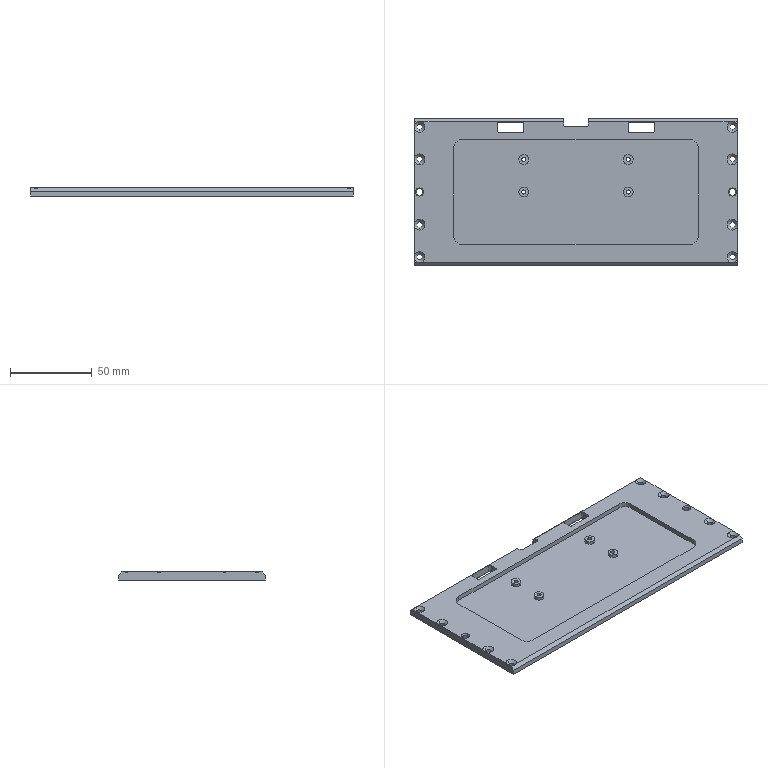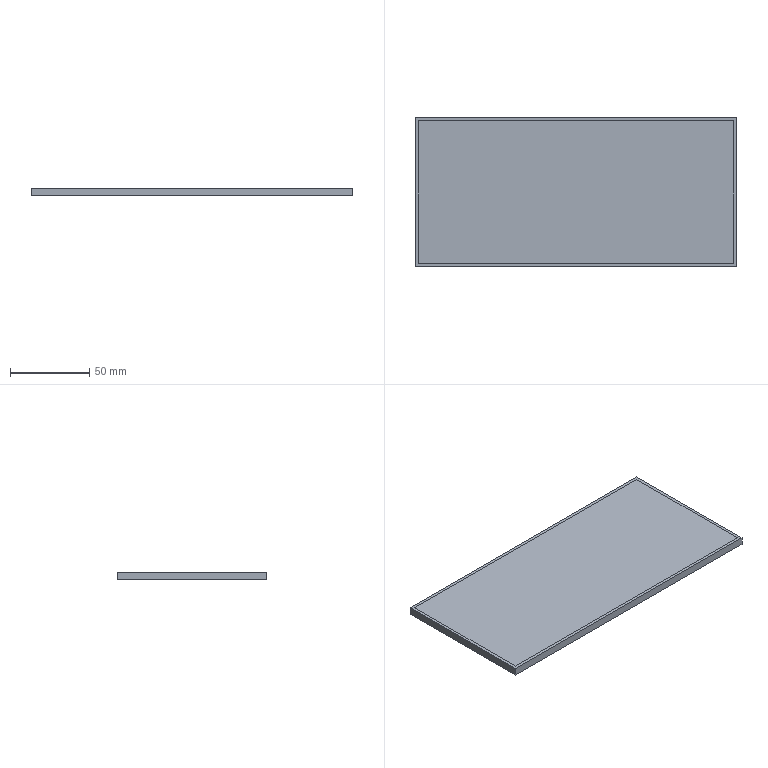CAM job | NX | 3-axis milling, drilling | part box 198 x 90 x 5 mm | stock box 202 x 94 x 5 mm
Tools:
number,name,description,diameter,corner_radius,flute_length,length,flutes
1,D6A45,Milling Tool-5 Parameters,6.0,0.0,50.0,75.0,2
16,3.4ZT,Drilling Tool,3.4,0.0,35.0,50.0,2
2,2.5ZT,Drilling Tool,2.5,0.0,35.0,50.0,2
15,D10,Milling Tool-5 Parameters,10.0,0.0,50.0,75.0,2
14,D10JING,Milling Tool-5 Parameters,10.0,0.0,50.0,75.0,2
11,D4,Milling Tool-5 Parameters,4.0,0.0,50.0,75.0,2
17,D2,Milling Tool-5 Parameters,2.0,0.0,50.0,75.0,2
12,D6,Milling Tool-5 Parameters,6.0,0.0,50.0,75.0,2
Operations:
program,operation,operation_type,tool,method,geometry_group,spindle_rpm,surface_speed,feed_per_tooth,feed_cut,feed_plunge,cut_length_mm,path_length_mm,cut_time_min,machine_time_min
1,DRILLING,Operation,D6A45,METHOD,A,5000.0,94.0,0.035,350.0,0.0,11.0,277.023,0.0314,0.058
1,DRILLING_COPY_COPY,Operation,D6A45,METHOD,A,5000.0,94.0,0.035,350.0,0.0,48.0,588.876,0.1371,0.1912
1,DRILLING_COPY_1_COPY,Operation,3.4ZT,METHOD,A,2000.0,21.0,0.05,200.0,0.0,76.172,586.486,0.3809,0.4319
1,DRILLING_COPY_1_COPY_COPY,Operation,2.5ZT,METHOD,A,2000.0,21.0,0.05,200.0,0.0,37.004,250.575,0.185,0.2064
1,ZLEVEL_PROFILE_COPY_1_COPY,ZLevelMilling,D10,METHOD,A,9500.0,298.0,0.1579,3000.0,1000.0,5563.553,5624.953,1.881,1.887
1,FLOOR_WALL,VolumeBased25DMillingOperation,D10,METHOD,A,9500.0,298.0,0.1579,3000.0,1000.0,4645.715,4756.622,1.643,1.654
1,FLOOR_WALL_COPY_1,VolumeBased25DMillingOperation,D10,METHOD,A,9500.0,298.0,0.1579,3000.0,1000.0,138.929,485.24,0.0675,0.1021
1,FLOOR_WALL_COPY,VolumeBased25DMillingOperation,D6,METHOD,A,9500.0,298.0,0.0789,1500.0,1000.0,3745.744,5253.795,2.51,2.66
1,ZLEVEL_PROFILE_COPY_1_COPY_COPY,ZLevelMilling,D4,METHOD,A,9500.0,119.0,0.1053,2000.0,1000.0,881.333,1080.405,0.4767,0.4966
1,ZLEVEL_PROFILE_COPY_1_COPY_COPY_COPY_COPY,ZLevelMilling,D2,METHOD,A,9500.0,59.0,0.0579,1100.0,1000.0,418.064,798.595,0.3825,0.4206
1,ZLEVEL_PROFILE_COPY_1_COPY_COPY_COPY,ZLevelMilling,D2,METHOD,A,9500.0,59.0,0.0579,1100.0,1000.0,681.695,1621.511,0.6298,0.7238
1,HOLE_MILLING,CylinderMilling,D2,METHOD,A,9500.0,59.0,0.0579,1100.0,100.0,431.801,752.801,0.3925,0.4246
1,ZLEVEL_PROFILE_COPY_1_COPY_COPY_COPY_1,ZLevelMilling,D6A45,METHOD,A,9500.0,179.0,0.0684,1300.0,1000.0,936.832,1802.172,0.7877,0.8742
1,PLANAR_MILL_COPY_COPY_COPY_COPY_COPY,PlanarMilling,D6A45,METHOD,A,9500.0,179.0,0.0658,1250.0,100.0,1100.075,1531.213,0.8801,0.9232
1,PLANAR_MILL_COPY_COPY_COPY_COPY_COPY_COPY,PlanarMilling,D6A45,METHOD,A,9500.0,179.0,0.0658,1250.0,100.0,143.381,753.587,0.1147,0.1757
1,PLANAR_MILL_COPY_COPY_COPY_COPY_COPY_COPY_1,PlanarMilling,D6A45,METHOD,A,9500.0,179.0,0.0658,1250.0,100.0,1218.566,2483.505,0.9749,1.101
1,CUTTERCOMP17,CylinderMilling,D2,METHOD,A,9500.0,59.0,0.0579,1100.0,100.0,52.572,373.572,0.0478,0.0799
1,ZLEVEL_PROFILE_COPY_1_COPY_COPY_1,ZLevelMilling,D10JING,METHOD,A,9500.0,298.0,0.0632,1200.0,1000.0,3072.901,3140.326,2.561,2.568
2,PLANAR_MILL_COPY_COPY_COPY_COPY_COPY_COPY_2,PlanarMilling,D6A45,METHOD,B,9500.0,179.0,0.0658,1250.0,100.0,858.876,2323.642,0.6871,0.8336
2,PLANAR_MILL_COPY_COPY_COPY_COPY_COPY_COPY_1_1,PlanarMilling,D6A45,METHOD,B,9500.0,179.0,0.0658,1250.0,100.0,83.789,283.853,0.067,0.087